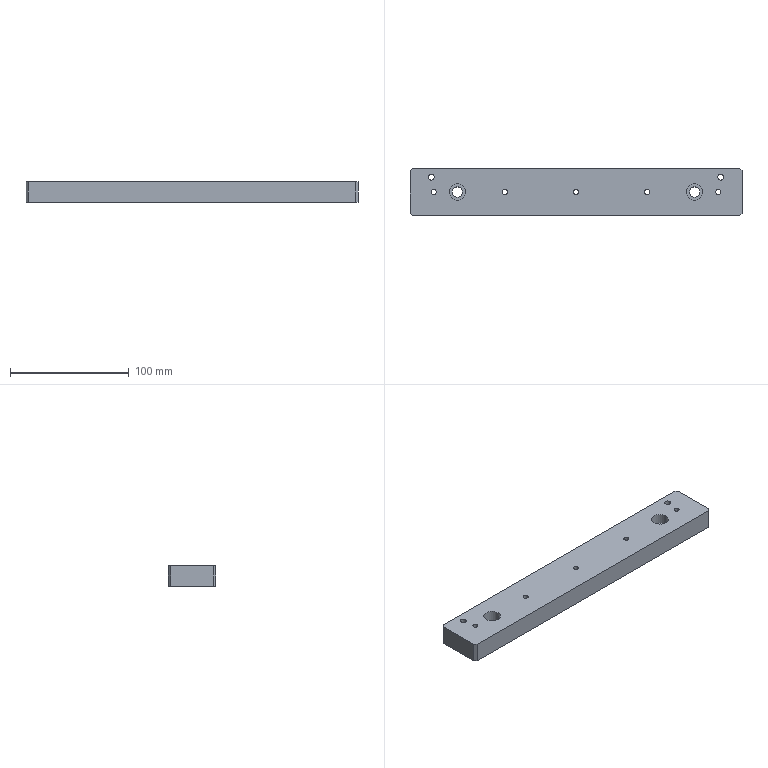Part | SolidWorks | features BaseBody 1 | 1 solid | 34 faces | box 280 x 40 x 17 mm | volume 184740 mm3 | cylinder 22 | plane 12 | commonest cylinder face diameters 4.2 x10 5 x4 8.5 x4 14 x4
STEP:
#1=CARTESIAN_POINT('',(-122.1,0.,0.));
#2=VERTEX_POINT('',#1);
#3=CARTESIAN_POINT('',(-117.9,0.,0.));
#4=VERTEX_POINT('',#3);
#5=CARTESIAN_POINT('',(-120.,0.,0.));
#6=DIRECTION('',(0.,0.,1.));
#7=DIRECTION('',(1.,0.,0.));
#8=AXIS2_PLACEMENT_3D('',#5,#6,#7);
#9=CIRCLE('',#8,2.1);
#10=EDGE_CURVE('',#2,#4,#9,.T.);
#11=ORIENTED_EDGE('',*,*,#10,.F.);
#12=CARTESIAN_POINT('',(-122.1,0.,17.));
#13=VERTEX_POINT('',#12);
#14=CARTESIAN_POINT('',(-122.1,0.,17.));
#15=DIRECTION('',(0.,0.,1.));
#16=VECTOR('',#15,1000.);
#17=LINE('',#14,#16);
#18=EDGE_CURVE('',#2,#13,#17,.T.);
#19=ORIENTED_EDGE('',*,*,#18,.T.);
#20=CARTESIAN_POINT('',(-117.9,0.,17.));
#21=VERTEX_POINT('',#20);
#22=CARTESIAN_POINT('',(-120.,0.,17.));
#23=DIRECTION('',(0.,0.,1.));
#24=DIRECTION('',(1.,0.,0.));
#25=AXIS2_PLACEMENT_3D('',#22,#23,#24);
#26=CIRCLE('',#25,2.1);
#27=EDGE_CURVE('',#13,#21,#26,.T.);
#28=ORIENTED_EDGE('',*,*,#27,.T.);
#29=CARTESIAN_POINT('',(-117.9,0.,17.));
#30=DIRECTION('',(0.,0.,1.));
#31=VECTOR('',#30,1000.);
#32=LINE('',#29,#31);
#33=EDGE_CURVE('',#4,#21,#32,.T.);
#34=ORIENTED_EDGE('',*,*,#33,.F.);
#35=EDGE_LOOP('',(#11,#19,#28,#34));
#36=FACE_OUTER_BOUND('',#35,.T.);
#37=CARTESIAN_POINT('',(-120.,0.,17.));
#38=DIRECTION('',(0.,0.,1.));
#39=DIRECTION('',(1.,0.,0.));
#40=AXIS2_PLACEMENT_3D('',#37,#38,#39);
#41=CYLINDRICAL_SURFACE('',#40,2.1);
#42=ADVANCED_FACE('',(#36),#41,.F.);
#43=CARTESIAN_POINT('',(-62.1,0.,0.));
#44=VERTEX_POINT('',#43);
#45=CARTESIAN_POINT('',(-57.9,0.,0.));
#46=VERTEX_POINT('',#45);
#47=CARTESIAN_POINT('',(-60.,0.,0.));
#48=DIRECTION('',(0.,0.,1.));
#49=DIRECTION('',(1.,0.,0.));
#50=AXIS2_PLACEMENT_3D('',#47,#48,#49);
#51=CIRCLE('',#50,2.1);
#52=EDGE_CURVE('',#44,#46,#51,.T.);
#53=ORIENTED_EDGE('',*,*,#52,.F.);
#54=CARTESIAN_POINT('',(-62.1,0.,17.));
#55=VERTEX_POINT('',#54);
#56=CARTESIAN_POINT('',(-62.1,0.,17.));
#57=DIRECTION('',(0.,0.,1.));
#58=VECTOR('',#57,1000.);
#59=LINE('',#56,#58);
#60=EDGE_CURVE('',#44,#55,#59,.T.);
#61=ORIENTED_EDGE('',*,*,#60,.T.);
#62=CARTESIAN_POINT('',(-57.9,0.,17.));
#63=VERTEX_POINT('',#62);
#64=CARTESIAN_POINT('',(-60.,0.,17.));
#65=DIRECTION('',(0.,0.,1.));
#66=DIRECTION('',(1.,0.,0.));
#67=AXIS2_PLACEMENT_3D('',#64,#65,#66);
#68=CIRCLE('',#67,2.1);
#69=EDGE_CURVE('',#55,#63,#68,.T.);
#70=ORIENTED_EDGE('',*,*,#69,.T.);
#71=CARTESIAN_POINT('',(-57.9,0.,17.));
#72=DIRECTION('',(0.,0.,1.));
#73=VECTOR('',#72,1000.);
#74=LINE('',#71,#73);
#75=EDGE_CURVE('',#46,#63,#74,.T.);
#76=ORIENTED_EDGE('',*,*,#75,.F.);
#77=EDGE_LOOP('',(#53,#61,#70,#76));
#78=FACE_OUTER_BOUND('',#77,.T.);
#79=CARTESIAN_POINT('',(-60.,0.,17.));
#80=DIRECTION('',(0.,0.,1.));
#81=DIRECTION('',(1.,0.,0.));
#82=AXIS2_PLACEMENT_3D('',#79,#80,#81);
#83=CYLINDRICAL_SURFACE('',#82,2.1);
#84=ADVANCED_FACE('',(#78),#83,.F.);
#85=CARTESIAN_POINT('',(-2.1,0.,0.));
#86=VERTEX_POINT('',#85);
#87=CARTESIAN_POINT('',(2.1,0.,0.));
#88=VERTEX_POINT('',#87);
#89=CARTESIAN_POINT('',(0.,0.,0.));
#90=DIRECTION('',(0.,0.,1.));
#91=DIRECTION('',(1.,0.,0.));
#92=AXIS2_PLACEMENT_3D('',#89,#90,#91);
#93=CIRCLE('',#92,2.1);
#94=EDGE_CURVE('',#86,#88,#93,.T.);
#95=ORIENTED_EDGE('',*,*,#94,.F.);
#96=CARTESIAN_POINT('',(-2.1,0.,17.));
#97=VERTEX_POINT('',#96);
#98=CARTESIAN_POINT('',(-2.1,0.,17.));
#99=DIRECTION('',(0.,0.,1.));
#100=VECTOR('',#99,1000.);
#101=LINE('',#98,#100);
#102=EDGE_CURVE('',#86,#97,#101,.T.);
#103=ORIENTED_EDGE('',*,*,#102,.T.);
#104=CARTESIAN_POINT('',(2.1,0.,17.));
#105=VERTEX_POINT('',#104);
#106=CARTESIAN_POINT('',(0.,0.,17.));
#107=DIRECTION('',(0.,0.,1.));
#108=DIRECTION('',(1.,0.,0.));
#109=AXIS2_PLACEMENT_3D('',#106,#107,#108);
#110=CIRCLE('',#109,2.1);
#111=EDGE_CURVE('',#97,#105,#110,.T.);
#112=ORIENTED_EDGE('',*,*,#111,.T.);
#113=CARTESIAN_POINT('',(2.1,0.,17.));
#114=DIRECTION('',(0.,0.,1.));
#115=VECTOR('',#114,1000.);
#116=LINE('',#113,#115);
#117=EDGE_CURVE('',#88,#105,#116,.T.);
#118=ORIENTED_EDGE('',*,*,#117,.F.);
#119=EDGE_LOOP('',(#95,#103,#112,#118));
#120=FACE_OUTER_BOUND('',#119,.T.);
#121=CARTESIAN_POINT('',(0.,0.,17.));
#122=DIRECTION('',(0.,0.,1.));
#123=DIRECTION('',(1.,0.,0.));
#124=AXIS2_PLACEMENT_3D('',#121,#122,#123);
#125=CYLINDRICAL_SURFACE('',#124,2.1);
#126=ADVANCED_FACE('',(#120),#125,.F.);
#127=CARTESIAN_POINT('',(57.9,0.,0.));
#128=VERTEX_POINT('',#127);
#129=CARTESIAN_POINT('',(62.1,0.,0.));
#130=VERTEX_POINT('',#129);
#131=CARTESIAN_POINT('',(60.,0.,0.));
#132=DIRECTION('',(0.,0.,1.));
#133=DIRECTION('',(1.,0.,0.));
#134=AXIS2_PLACEMENT_3D('',#131,#132,#133);
#135=CIRCLE('',#134,2.1);
#136=EDGE_CURVE('',#128,#130,#135,.T.);
#137=ORIENTED_EDGE('',*,*,#136,.F.);
#138=CARTESIAN_POINT('',(57.9,0.,17.));
#139=VERTEX_POINT('',#138);
#140=CARTESIAN_POINT('',(57.9,0.,17.));
#141=DIRECTION('',(0.,0.,1.));
#142=VECTOR('',#141,1000.);
#143=LINE('',#140,#142);
#144=EDGE_CURVE('',#128,#139,#143,.T.);
#145=ORIENTED_EDGE('',*,*,#144,.T.);
#146=CARTESIAN_POINT('',(62.1,0.,17.));
#147=VERTEX_POINT('',#146);
#148=CARTESIAN_POINT('',(60.,0.,17.));
#149=DIRECTION('',(0.,0.,1.));
#150=DIRECTION('',(1.,0.,0.));
#151=AXIS2_PLACEMENT_3D('',#148,#149,#150);
#152=CIRCLE('',#151,2.1);
#153=EDGE_CURVE('',#139,#147,#152,.T.);
#154=ORIENTED_EDGE('',*,*,#153,.T.);
#155=CARTESIAN_POINT('',(62.1,0.,17.));
#156=DIRECTION('',(0.,0.,1.));
#157=VECTOR('',#156,1000.);
#158=LINE('',#155,#157);
#159=EDGE_CURVE('',#130,#147,#158,.T.);
#160=ORIENTED_EDGE('',*,*,#159,.F.);
#161=EDGE_LOOP('',(#137,#145,#154,#160));
#162=FACE_OUTER_BOUND('',#161,.T.);
#163=CARTESIAN_POINT('',(60.,0.,17.));
#164=DIRECTION('',(0.,0.,1.));
#165=DIRECTION('',(1.,0.,0.));
#166=AXIS2_PLACEMENT_3D('',#163,#164,#165);
#167=CYLINDRICAL_SURFACE('',#166,2.1);
#168=ADVANCED_FACE('',(#162),#167,.F.);
#169=CARTESIAN_POINT('',(117.9,0.,0.));
#170=VERTEX_POINT('',#169);
#171=CARTESIAN_POINT('',(122.1,0.,0.));
#172=VERTEX_POINT('',#171);
#173=CARTESIAN_POINT('',(120.,0.,0.));
#174=DIRECTION('',(0.,0.,1.));
#175=DIRECTION('',(1.,0.,0.));
#176=AXIS2_PLACEMENT_3D('',#173,#174,#175);
#177=CIRCLE('',#176,2.1);
#178=EDGE_CURVE('',#170,#172,#177,.T.);
#179=ORIENTED_EDGE('',*,*,#178,.F.);
#180=CARTESIAN_POINT('',(117.9,0.,17.));
#181=VERTEX_POINT('',#180);
#182=CARTESIAN_POINT('',(117.9,0.,17.));
#183=DIRECTION('',(0.,0.,1.));
#184=VECTOR('',#183,1000.);
#185=LINE('',#182,#184);
#186=EDGE_CURVE('',#170,#181,#185,.T.);
#187=ORIENTED_EDGE('',*,*,#186,.T.);
#188=CARTESIAN_POINT('',(122.1,0.,17.));
#189=VERTEX_POINT('',#188);
#190=CARTESIAN_POINT('',(120.,0.,17.));
#191=DIRECTION('',(0.,0.,1.));
#192=DIRECTION('',(1.,0.,0.));
#193=AXIS2_PLACEMENT_3D('',#190,#191,#192);
#194=CIRCLE('',#193,2.1);
#195=EDGE_CURVE('',#181,#189,#194,.T.);
#196=ORIENTED_EDGE('',*,*,#195,.T.);
#197=CARTESIAN_POINT('',(122.1,0.,17.));
#198=DIRECTION('',(0.,0.,1.));
#199=VECTOR('',#198,1000.);
#200=LINE('',#197,#199);
#201=EDGE_CURVE('',#172,#189,#200,.T.);
#202=ORIENTED_EDGE('',*,*,#201,.F.);
#203=EDGE_LOOP('',(#179,#187,#196,#202));
#204=FACE_OUTER_BOUND('',#203,.T.);
#205=CARTESIAN_POINT('',(120.,0.,17.));
#206=DIRECTION('',(0.,0.,1.));
#207=DIRECTION('',(1.,0.,0.));
#208=AXIS2_PLACEMENT_3D('',#205,#206,#207);
#209=CYLINDRICAL_SURFACE('',#208,2.1);
#210=ADVANCED_FACE('',(#204),#209,.F.);
#211=CARTESIAN_POINT('',(-119.5,12.5,0.));
#212=VERTEX_POINT('',#211);
#213=CARTESIAN_POINT('',(-124.5,12.5,0.));
#214=VERTEX_POINT('',#213);
#215=CARTESIAN_POINT('',(-122.,12.5,0.));
#216=DIRECTION('',(0.,0.,-1.));
#217=DIRECTION('',(-1.,0.,0.));
#218=AXIS2_PLACEMENT_3D('',#215,#216,#217);
#219=CIRCLE('',#218,2.5);
#220=EDGE_CURVE('',#212,#214,#219,.T.);
#221=ORIENTED_EDGE('',*,*,#220,.T.);
#222=CARTESIAN_POINT('',(-124.5,12.5,17.));
#223=VERTEX_POINT('',#222);
#224=CARTESIAN_POINT('',(-124.5,12.5,17.));
#225=DIRECTION('',(0.,0.,1.));
#226=VECTOR('',#225,1000.);
#227=LINE('',#224,#226);
#228=EDGE_CURVE('',#214,#223,#227,.T.);
#229=ORIENTED_EDGE('',*,*,#228,.T.);
#230=CARTESIAN_POINT('',(-119.5,12.5,17.));
#231=VERTEX_POINT('',#230);
#232=CARTESIAN_POINT('',(-122.,12.5,17.));
#233=DIRECTION('',(0.,0.,1.));
#234=DIRECTION('',(1.,0.,0.));
#235=AXIS2_PLACEMENT_3D('',#232,#233,#234);
#236=CIRCLE('',#235,2.5);
#237=EDGE_CURVE('',#223,#231,#236,.T.);
#238=ORIENTED_EDGE('',*,*,#237,.T.);
#239=CARTESIAN_POINT('',(-119.5,12.5,17.));
#240=DIRECTION('',(0.,0.,1.));
#241=VECTOR('',#240,1000.);
#242=LINE('',#239,#241);
#243=EDGE_CURVE('',#212,#231,#242,.T.);
#244=ORIENTED_EDGE('',*,*,#243,.F.);
#245=EDGE_LOOP('',(#221,#229,#238,#244));
#246=FACE_OUTER_BOUND('',#245,.T.);
#247=CARTESIAN_POINT('',(-122.,12.5,17.));
#248=DIRECTION('',(0.,0.,1.));
#249=DIRECTION('',(1.,0.,0.));
#250=AXIS2_PLACEMENT_3D('',#247,#248,#249);
#251=CYLINDRICAL_SURFACE('',#250,2.5);
#252=ADVANCED_FACE('',(#246),#251,.F.);
#253=CARTESIAN_POINT('',(124.5,12.5,0.));
#254=VERTEX_POINT('',#253);
#255=CARTESIAN_POINT('',(119.5,12.5,0.));
#256=VERTEX_POINT('',#255);
#257=CARTESIAN_POINT('',(122.,12.5,0.));
#258=DIRECTION('',(0.,0.,-1.));
#259=DIRECTION('',(-1.,0.,0.));
#260=AXIS2_PLACEMENT_3D('',#257,#258,#259);
#261=CIRCLE('',#260,2.5);
#262=EDGE_CURVE('',#254,#256,#261,.T.);
#263=ORIENTED_EDGE('',*,*,#262,.T.);
#264=CARTESIAN_POINT('',(119.5,12.5,17.));
#265=VERTEX_POINT('',#264);
#266=CARTESIAN_POINT('',(119.5,12.5,17.));
#267=DIRECTION('',(0.,0.,1.));
#268=VECTOR('',#267,1000.);
#269=LINE('',#266,#268);
#270=EDGE_CURVE('',#256,#265,#269,.T.);
#271=ORIENTED_EDGE('',*,*,#270,.T.);
#272=CARTESIAN_POINT('',(124.5,12.5,17.));
#273=VERTEX_POINT('',#272);
#274=CARTESIAN_POINT('',(122.,12.5,17.));
#275=DIRECTION('',(0.,0.,1.));
#276=DIRECTION('',(1.,0.,0.));
#277=AXIS2_PLACEMENT_3D('',#274,#275,#276);
#278=CIRCLE('',#277,2.5);
#279=EDGE_CURVE('',#265,#273,#278,.T.);
#280=ORIENTED_EDGE('',*,*,#279,.T.);
#281=CARTESIAN_POINT('',(124.5,12.5,17.));
#282=DIRECTION('',(0.,0.,1.));
#283=VECTOR('',#282,1000.);
#284=LINE('',#281,#283);
#285=EDGE_CURVE('',#254,#273,#284,.T.);
#286=ORIENTED_EDGE('',*,*,#285,.F.);
#287=EDGE_LOOP('',(#263,#271,#280,#286));
#288=FACE_OUTER_BOUND('',#287,.T.);
#289=CARTESIAN_POINT('',(122.,12.5,17.));
#290=DIRECTION('',(0.,0.,1.));
#291=DIRECTION('',(1.,0.,0.));
#292=AXIS2_PLACEMENT_3D('',#289,#290,#291);
#293=CYLINDRICAL_SURFACE('',#292,2.5);
#294=ADVANCED_FACE('',(#288),#293,.F.);
#295=CARTESIAN_POINT('',(-107.,0.,8.));
#296=VERTEX_POINT('',#295);
#297=CARTESIAN_POINT('',(-93.,0.,8.));
#298=VERTEX_POINT('',#297);
#299=CARTESIAN_POINT('',(-100.,0.,8.));
#300=DIRECTION('',(0.,0.,1.));
#301=DIRECTION('',(1.,0.,0.));
#302=AXIS2_PLACEMENT_3D('',#299,#300,#301);
#303=CIRCLE('',#302,7.);
#304=EDGE_CURVE('',#296,#298,#303,.T.);
#305=ORIENTED_EDGE('',*,*,#304,.F.);
#306=CARTESIAN_POINT('',(-107.,0.,17.));
#307=VERTEX_POINT('',#306);
#308=CARTESIAN_POINT('',(-107.,0.,17.));
#309=DIRECTION('',(0.,0.,1.));
#310=VECTOR('',#309,1000.);
#311=LINE('',#308,#310);
#312=EDGE_CURVE('',#296,#307,#311,.T.);
#313=ORIENTED_EDGE('',*,*,#312,.T.);
#314=CARTESIAN_POINT('',(-93.,0.,17.));
#315=VERTEX_POINT('',#314);
#316=CARTESIAN_POINT('',(-100.,0.,17.));
#317=DIRECTION('',(0.,0.,1.));
#318=DIRECTION('',(1.,0.,0.));
#319=AXIS2_PLACEMENT_3D('',#316,#317,#318);
#320=CIRCLE('',#319,7.);
#321=EDGE_CURVE('',#307,#315,#320,.T.);
#322=ORIENTED_EDGE('',*,*,#321,.T.);
#323=CARTESIAN_POINT('',(-93.,0.,17.));
#324=DIRECTION('',(0.,0.,1.));
#325=VECTOR('',#324,1000.);
#326=LINE('',#323,#325);
#327=EDGE_CURVE('',#298,#315,#326,.T.);
#328=ORIENTED_EDGE('',*,*,#327,.F.);
#329=EDGE_LOOP('',(#305,#313,#322,#328));
#330=FACE_OUTER_BOUND('',#329,.T.);
#331=CARTESIAN_POINT('',(-100.,0.,17.));
#332=DIRECTION('',(0.,0.,1.));
#333=DIRECTION('',(1.,0.,0.));
#334=AXIS2_PLACEMENT_3D('',#331,#332,#333);
#335=CYLINDRICAL_SURFACE('',#334,7.);
#336=ADVANCED_FACE('',(#330),#335,.F.);
#337=CARTESIAN_POINT('',(-104.25,0.,0.));
#338=VERTEX_POINT('',#337);
#339=CARTESIAN_POINT('',(-95.75,0.,0.));
#340=VERTEX_POINT('',#339);
#341=CARTESIAN_POINT('',(-100.,0.,0.));
#342=DIRECTION('',(0.,0.,1.));
#343=DIRECTION('',(1.,0.,0.));
#344=AXIS2_PLACEMENT_3D('',#341,#342,#343);
#345=CIRCLE('',#344,4.25);
#346=EDGE_CURVE('',#338,#340,#345,.T.);
#347=ORIENTED_EDGE('',*,*,#346,.F.);
#348=CARTESIAN_POINT('',(-104.25,0.,8.));
#349=VERTEX_POINT('',#348);
#350=CARTESIAN_POINT('',(-104.25,0.,17.));
#351=DIRECTION('',(0.,0.,1.));
#352=VECTOR('',#351,1000.);
#353=LINE('',#350,#352);
#354=EDGE_CURVE('',#338,#349,#353,.T.);
#355=ORIENTED_EDGE('',*,*,#354,.T.);
#356=CARTESIAN_POINT('',(-95.75,0.,8.));
#357=VERTEX_POINT('',#356);
#358=CARTESIAN_POINT('',(-100.,0.,8.));
#359=DIRECTION('',(0.,0.,1.));
#360=DIRECTION('',(1.,0.,0.));
#361=AXIS2_PLACEMENT_3D('',#358,#359,#360);
#362=CIRCLE('',#361,4.25);
#363=EDGE_CURVE('',#349,#357,#362,.T.);
#364=ORIENTED_EDGE('',*,*,#363,.T.);
#365=CARTESIAN_POINT('',(-95.75,0.,17.));
#366=DIRECTION('',(0.,0.,1.));
#367=VECTOR('',#366,1000.);
#368=LINE('',#365,#367);
#369=EDGE_CURVE('',#340,#357,#368,.T.);
#370=ORIENTED_EDGE('',*,*,#369,.F.);
#371=EDGE_LOOP('',(#347,#355,#364,#370));
#372=FACE_OUTER_BOUND('',#371,.T.);
#373=CARTESIAN_POINT('',(-100.,0.,17.));
#374=DIRECTION('',(0.,0.,1.));
#375=DIRECTION('',(1.,0.,0.));
#376=AXIS2_PLACEMENT_3D('',#373,#374,#375);
#377=CYLINDRICAL_SURFACE('',#376,4.25);
#378=ADVANCED_FACE('',(#372),#377,.F.);
#379=CARTESIAN_POINT('',(93.,0.,8.));
#380=VERTEX_POINT('',#379);
#381=CARTESIAN_POINT('',(107.,0.,8.));
#382=VERTEX_POINT('',#381);
#383=CARTESIAN_POINT('',(100.,0.,8.));
#384=DIRECTION('',(0.,0.,1.));
#385=DIRECTION('',(1.,0.,0.));
#386=AXIS2_PLACEMENT_3D('',#383,#384,#385);
#387=CIRCLE('',#386,7.);
#388=EDGE_CURVE('',#380,#382,#387,.T.);
#389=ORIENTED_EDGE('',*,*,#388,.F.);
#390=CARTESIAN_POINT('',(93.,0.,17.));
#391=VERTEX_POINT('',#390);
#392=CARTESIAN_POINT('',(93.,0.,17.));
#393=DIRECTION('',(0.,0.,1.));
#394=VECTOR('',#393,1000.);
#395=LINE('',#392,#394);
#396=EDGE_CURVE('',#380,#391,#395,.T.);
#397=ORIENTED_EDGE('',*,*,#396,.T.);
#398=CARTESIAN_POINT('',(107.,0.,17.));
#399=VERTEX_POINT('',#398);
#400=CARTESIAN_POINT('',(100.,0.,17.));
#401=DIRECTION('',(0.,0.,1.));
#402=DIRECTION('',(1.,0.,0.));
#403=AXIS2_PLACEMENT_3D('',#400,#401,#402);
#404=CIRCLE('',#403,7.);
#405=EDGE_CURVE('',#391,#399,#404,.T.);
#406=ORIENTED_EDGE('',*,*,#405,.T.);
#407=CARTESIAN_POINT('',(107.,0.,17.));
#408=DIRECTION('',(0.,0.,1.));
#409=VECTOR('',#408,1000.);
#410=LINE('',#407,#409);
#411=EDGE_CURVE('',#382,#399,#410,.T.);
#412=ORIENTED_EDGE('',*,*,#411,.F.);
#413=EDGE_LOOP('',(#389,#397,#406,#412));
#414=FACE_OUTER_BOUND('',#413,.T.);
#415=CARTESIAN_POINT('',(100.,0.,17.));
#416=DIRECTION('',(0.,0.,1.));
#417=DIRECTION('',(1.,0.,0.));
#418=AXIS2_PLACEMENT_3D('',#415,#416,#417);
#419=CYLINDRICAL_SURFACE('',#418,7.);
#420=ADVANCED_FACE('',(#414),#419,.F.);
#421=CARTESIAN_POINT('',(95.75,0.,0.));
#422=VERTEX_POINT('',#421);
#423=CARTESIAN_POINT('',(104.25,0.,0.));
#424=VERTEX_POINT('',#423);
#425=CARTESIAN_POINT('',(100.,0.,0.));
#426=DIRECTION('',(0.,0.,1.));
#427=DIRECTION('',(1.,0.,0.));
#428=AXIS2_PLACEMENT_3D('',#425,#426,#427);
#429=CIRCLE('',#428,4.25);
#430=EDGE_CURVE('',#422,#424,#429,.T.);
#431=ORIENTED_EDGE('',*,*,#430,.F.);
#432=CARTESIAN_POINT('',(95.75,0.,8.));
#433=VERTEX_POINT('',#432);
#434=CARTESIAN_POINT('',(95.75,0.,17.));
#435=DIRECTION('',(0.,0.,1.));
#436=VECTOR('',#435,1000.);
#437=LINE('',#434,#436);
#438=EDGE_CURVE('',#422,#433,#437,.T.);
#439=ORIENTED_EDGE('',*,*,#438,.T.);
#440=CARTESIAN_POINT('',(104.25,0.,8.));
#441=VERTEX_POINT('',#440);
#442=CARTESIAN_POINT('',(100.,0.,8.));
#443=DIRECTION('',(0.,0.,1.));
#444=DIRECTION('',(1.,0.,0.));
#445=AXIS2_PLACEMENT_3D('',#442,#443,#444);
#446=CIRCLE('',#445,4.25);
#447=EDGE_CURVE('',#433,#441,#446,.T.);
#448=ORIENTED_EDGE('',*,*,#447,.T.);
#449=CARTESIAN_POINT('',(104.25,0.,17.));
#450=DIRECTION('',(0.,0.,1.));
#451=VECTOR('',#450,1000.);
#452=LINE('',#449,#451);
#453=EDGE_CURVE('',#424,#441,#452,.T.);
#454=ORIENTED_EDGE('',*,*,#453,.F.);
#455=EDGE_LOOP('',(#431,#439,#448,#454));
#456=FACE_OUTER_BOUND('',#455,.T.);
#457=CARTESIAN_POINT('',(100.,0.,17.));
#458=DIRECTION('',(0.,0.,1.));
#459=DIRECTION('',(1.,0.,0.));
#460=AXIS2_PLACEMENT_3D('',#457,#458,#459);
#461=CYLINDRICAL_SURFACE('',#460,4.25);
#462=ADVANCED_FACE('',(#456),#461,.F.);
#463=CARTESIAN_POINT('',(-140.,18.,17.));
#464=VERTEX_POINT('',#463);
#465=CARTESIAN_POINT('',(-140.,-18.,17.));
#466=VERTEX_POINT('',#465);
#467=CARTESIAN_POINT('',(-140.,20.,17.));
#468=DIRECTION('',(0.,-1.,0.));
#469=VECTOR('',#468,1000.);
#470=LINE('',#467,#469);
#471=EDGE_CURVE('',#464,#466,#470,.T.);
#472=ORIENTED_EDGE('',*,*,#471,.F.);
#473=CARTESIAN_POINT('',(-140.,18.,0.));
#474=VERTEX_POINT('',#473);
#475=CARTESIAN_POINT('',(-140.,18.,17.));
#476=DIRECTION('',(0.,0.,-1.));
#477=VECTOR('',#476,1000.);
#478=LINE('',#475,#477);
#479=EDGE_CURVE('',#464,#474,#478,.T.);
#480=ORIENTED_EDGE('',*,*,#479,.T.);
#481=CARTESIAN_POINT('',(-140.,-18.,0.));
#482=VERTEX_POINT('',#481);
#483=CARTESIAN_POINT('',(-140.,20.,0.));
#484=DIRECTION('',(0.,-1.,0.));
#485=VECTOR('',#484,1000.);
#486=LINE('',#483,#485);
#487=EDGE_CURVE('',#474,#482,#486,.T.);
#488=ORIENTED_EDGE('',*,*,#487,.T.);
#489=CARTESIAN_POINT('',(-140.,-18.,17.));
#490=DIRECTION('',(0.,0.,1.));
#491=VECTOR('',#490,1000.);
#492=LINE('',#489,#491);
#493=EDGE_CURVE('',#482,#466,#492,.T.);
#494=ORIENTED_EDGE('',*,*,#493,.T.);
#495=EDGE_LOOP('',(#472,#480,#488,#494));
#496=FACE_OUTER_BOUND('',#495,.T.);
#497=CARTESIAN_POINT('',(-140.,20.,17.));
#498=DIRECTION('',(1.,0.,0.));
#499=DIRECTION('',(0.,0.,-1.));
#500=AXIS2_PLACEMENT_3D('',#497,#498,#499);
#501=PLANE('',#500);
#502=ADVANCED_FACE('',(#496),#501,.F.);
#503=CARTESIAN_POINT('',(-138.,-20.,0.));
#504=VERTEX_POINT('',#503);
#505=CARTESIAN_POINT('',(138.,-20.,0.));
#506=VERTEX_POINT('',#505);
#507=CARTESIAN_POINT('',(140.,-20.,0.));
#508=DIRECTION('',(1.,0.,0.));
#509=VECTOR('',#508,1000.);
#510=LINE('',#507,#509);
#511=EDGE_CURVE('',#504,#506,#510,.T.);
#512=ORIENTED_EDGE('',*,*,#511,.T.);
#513=CARTESIAN_POINT('',(138.,-20.,17.));
#514=VERTEX_POINT('',#513);
#515=CARTESIAN_POINT('',(138.,-20.,17.));
#516=DIRECTION('',(0.,0.,1.));
#517=VECTOR('',#516,1000.);
#518=LINE('',#515,#517);
#519=EDGE_CURVE('',#506,#514,#518,.T.);
#520=ORIENTED_EDGE('',*,*,#519,.T.);
#521=CARTESIAN_POINT('',(-138.,-20.,17.));
#522=VERTEX_POINT('',#521);
#523=CARTESIAN_POINT('',(140.,-20.,17.));
#524=DIRECTION('',(1.,0.,0.));
#525=VECTOR('',#524,1000.);
#526=LINE('',#523,#525);
#527=EDGE_CURVE('',#522,#514,#526,.T.);
#528=ORIENTED_EDGE('',*,*,#527,.F.);
#529=CARTESIAN_POINT('',(-138.,-20.,17.));
#530=DIRECTION('',(0.,0.,-1.));
#531=VECTOR('',#530,1000.);
#532=LINE('',#529,#531);
#533=EDGE_CURVE('',#522,#504,#532,.T.);
#534=ORIENTED_EDGE('',*,*,#533,.T.);
#535=EDGE_LOOP('',(#512,#520,#528,#534));
#536=FACE_OUTER_BOUND('',#535,.T.);
#537=CARTESIAN_POINT('',(140.,-20.,17.));
#538=DIRECTION('',(0.,1.,0.));
#539=DIRECTION('',(-1.,0.,0.));
#540=AXIS2_PLACEMENT_3D('',#537,#538,#539);
#541=PLANE('',#540);
#542=ADVANCED_FACE('',(#536),#541,.F.);
#543=CARTESIAN_POINT('',(140.,-18.,17.));
#544=VERTEX_POINT('',#543);
#545=CARTESIAN_POINT('',(140.,18.,17.));
#546=VERTEX_POINT('',#545);
#547=CARTESIAN_POINT('',(140.,20.,17.));
#548=DIRECTION('',(0.,1.,0.));
#549=VECTOR('',#548,1000.);
#550=LINE('',#547,#549);
#551=EDGE_CURVE('',#544,#546,#550,.T.);
#552=ORIENTED_EDGE('',*,*,#551,.F.);
#553=CARTESIAN_POINT('',(140.,-18.,0.));
#554=VERTEX_POINT('',#553);
#555=CARTESIAN_POINT('',(140.,-18.,17.));
#556=DIRECTION('',(0.,0.,-1.));
#557=VECTOR('',#556,1000.);
#558=LINE('',#555,#557);
#559=EDGE_CURVE('',#544,#554,#558,.T.);
#560=ORIENTED_EDGE('',*,*,#559,.T.);
#561=CARTESIAN_POINT('',(140.,18.,0.));
#562=VERTEX_POINT('',#561);
#563=CARTESIAN_POINT('',(140.,20.,0.));
#564=DIRECTION('',(0.,1.,0.));
#565=VECTOR('',#564,1000.);
#566=LINE('',#563,#565);
#567=EDGE_CURVE('',#554,#562,#566,.T.);
#568=ORIENTED_EDGE('',*,*,#567,.T.);
#569=CARTESIAN_POINT('',(140.,18.,17.));
#570=DIRECTION('',(0.,0.,1.));
#571=VECTOR('',#570,1000.);
#572=LINE('',#569,#571);
#573=EDGE_CURVE('',#562,#546,#572,.T.);
#574=ORIENTED_EDGE('',*,*,#573,.T.);
#575=EDGE_LOOP('',(#552,#560,#568,#574));
#576=FACE_OUTER_BOUND('',#575,.T.);
#577=CARTESIAN_POINT('',(140.,20.,17.));
#578=DIRECTION('',(-1.,0.,0.));
#579=DIRECTION('',(0.,0.,1.));
#580=AXIS2_PLACEMENT_3D('',#577,#578,#579);
#581=PLANE('',#580);
#582=ADVANCED_FACE('',(#576),#581,.F.);
#583=CARTESIAN_POINT('',(138.,20.,17.));
#584=VERTEX_POINT('',#583);
#585=CARTESIAN_POINT('',(-138.,20.,17.));
#586=VERTEX_POINT('',#585);
#587=CARTESIAN_POINT('',(140.,20.,17.));
#588=DIRECTION('',(-1.,0.,0.));
#589=VECTOR('',#588,1000.);
#590=LINE('',#587,#589);
#591=EDGE_CURVE('',#584,#586,#590,.T.);
#592=ORIENTED_EDGE('',*,*,#591,.F.);
#593=CARTESIAN_POINT('',(138.,20.,0.));
#594=VERTEX_POINT('',#593);
#595=CARTESIAN_POINT('',(138.,20.,17.));
#596=DIRECTION('',(0.,0.,-1.));
#597=VECTOR('',#596,1000.);
#598=LINE('',#595,#597);
#599=EDGE_CURVE('',#584,#594,#598,.T.);
#600=ORIENTED_EDGE('',*,*,#599,.T.);
#601=CARTESIAN_POINT('',(-138.,20.,0.));
#602=VERTEX_POINT('',#601);
#603=CARTESIAN_POINT('',(140.,20.,0.));
#604=DIRECTION('',(-1.,0.,0.));
#605=VECTOR('',#604,1000.);
#606=LINE('',#603,#605);
#607=EDGE_CURVE('',#594,#602,#606,.T.);
#608=ORIENTED_EDGE('',*,*,#607,.T.);
#609=CARTESIAN_POINT('',(-138.,20.,17.));
#610=DIRECTION('',(0.,0.,1.));
#611=VECTOR('',#610,1000.);
#612=LINE('',#609,#611);
#613=EDGE_CURVE('',#602,#586,#612,.T.);
#614=ORIENTED_EDGE('',*,*,#613,.T.);
#615=EDGE_LOOP('',(#592,#600,#608,#614));
#616=FACE_OUTER_BOUND('',#615,.T.);
#617=CARTESIAN_POINT('',(140.,20.,17.));
#618=DIRECTION('',(0.,-1.,0.));
#619=DIRECTION('',(1.,0.,0.));
#620=AXIS2_PLACEMENT_3D('',#617,#618,#619);
#621=PLANE('',#620);
#622=ADVANCED_FACE('',(#616),#621,.F.);
#623=CARTESIAN_POINT('',(-120.,0.,17.));
#624=DIRECTION('',(0.,0.,1.));
#625=DIRECTION('',(1.,0.,0.));
#626=AXIS2_PLACEMENT_3D('',#623,#624,#625);
#627=CIRCLE('',#626,2.1);
#628=EDGE_CURVE('',#21,#13,#627,.T.);
#629=ORIENTED_EDGE('',*,*,#628,.F.);
#630=ORIENTED_EDGE('',*,*,#27,.F.);
#631=EDGE_LOOP('',(#629,#630));
#632=FACE_BOUND('',#631,.T.);
#633=CARTESIAN_POINT('',(-60.,0.,17.));
#634=DIRECTION('',(0.,0.,1.));
#635=DIRECTION('',(1.,0.,0.));
#636=AXIS2_PLACEMENT_3D('',#633,#634,#635);
#637=CIRCLE('',#636,2.1);
#638=EDGE_CURVE('',#63,#55,#637,.T.);
#639=ORIENTED_EDGE('',*,*,#638,.F.);
#640=ORIENTED_EDGE('',*,*,#69,.F.);
#641=EDGE_LOOP('',(#639,#640));
#642=FACE_BOUND('',#641,.T.);
#643=CARTESIAN_POINT('',(0.,0.,17.));
#644=DIRECTION('',(0.,0.,1.));
#645=DIRECTION('',(1.,0.,0.));
#646=AXIS2_PLACEMENT_3D('',#643,#644,#645);
#647=CIRCLE('',#646,2.1);
#648=EDGE_CURVE('',#105,#97,#647,.T.);
#649=ORIENTED_EDGE('',*,*,#648,.F.);
#650=ORIENTED_EDGE('',*,*,#111,.F.);
#651=EDGE_LOOP('',(#649,#650));
#652=FACE_BOUND('',#651,.T.);
#653=CARTESIAN_POINT('',(60.,0.,17.));
#654=DIRECTION('',(0.,0.,1.));
#655=DIRECTION('',(1.,0.,0.));
#656=AXIS2_PLACEMENT_3D('',#653,#654,#655);
#657=CIRCLE('',#656,2.1);
#658=EDGE_CURVE('',#147,#139,#657,.T.);
#659=ORIENTED_EDGE('',*,*,#658,.F.);
#660=ORIENTED_EDGE('',*,*,#153,.F.);
#661=EDGE_LOOP('',(#659,#660));
#662=FACE_BOUND('',#661,.T.);
#663=CARTESIAN_POINT('',(120.,0.,17.));
#664=DIRECTION('',(0.,0.,1.));
#665=DIRECTION('',(1.,0.,0.));
#666=AXIS2_PLACEMENT_3D('',#663,#664,#665);
#667=CIRCLE('',#666,2.1);
#668=EDGE_CURVE('',#189,#181,#667,.T.);
#669=ORIENTED_EDGE('',*,*,#668,.F.);
#670=ORIENTED_EDGE('',*,*,#195,.F.);
#671=EDGE_LOOP('',(#669,#670));
#672=FACE_BOUND('',#671,.T.);
#673=CARTESIAN_POINT('',(-122.,12.5,17.));
#674=DIRECTION('',(0.,0.,1.));
#675=DIRECTION('',(1.,0.,0.));
#676=AXIS2_PLACEMENT_3D('',#673,#674,#675);
#677=CIRCLE('',#676,2.5);
#678=EDGE_CURVE('',#231,#223,#677,.T.);
#679=ORIENTED_EDGE('',*,*,#678,.F.);
#680=ORIENTED_EDGE('',*,*,#237,.F.);
#681=EDGE_LOOP('',(#679,#680));
#682=FACE_BOUND('',#681,.T.);
#683=CARTESIAN_POINT('',(122.,12.5,17.));
#684=DIRECTION('',(0.,0.,1.));
#685=DIRECTION('',(1.,0.,0.));
#686=AXIS2_PLACEMENT_3D('',#683,#684,#685);
#687=CIRCLE('',#686,2.5);
#688=EDGE_CURVE('',#273,#265,#687,.T.);
#689=ORIENTED_EDGE('',*,*,#688,.F.);
#690=ORIENTED_EDGE('',*,*,#279,.F.);
#691=EDGE_LOOP('',(#689,#690));
#692=FACE_BOUND('',#691,.T.);
#693=CARTESIAN_POINT('',(-100.,0.,17.));
#694=DIRECTION('',(0.,0.,1.));
#695=DIRECTION('',(1.,0.,0.));
#696=AXIS2_PLACEMENT_3D('',#693,#694,#695);
#697=CIRCLE('',#696,7.);
#698=EDGE_CURVE('',#315,#307,#697,.T.);
#699=ORIENTED_EDGE('',*,*,#698,.F.);
#700=ORIENTED_EDGE('',*,*,#321,.F.);
#701=EDGE_LOOP('',(#699,#700));
#702=FACE_BOUND('',#701,.T.);
#703=CARTESIAN_POINT('',(100.,0.,17.));
#704=DIRECTION('',(0.,0.,1.));
#705=DIRECTION('',(1.,0.,0.));
#706=AXIS2_PLACEMENT_3D('',#703,#704,#705);
#707=CIRCLE('',#706,7.);
#708=EDGE_CURVE('',#399,#391,#707,.T.);
#709=ORIENTED_EDGE('',*,*,#708,.F.);
#710=ORIENTED_EDGE('',*,*,#405,.F.);
#711=EDGE_LOOP('',(#709,#710));
#712=FACE_BOUND('',#711,.T.);
#713=ORIENTED_EDGE('',*,*,#527,.T.);
#714=CARTESIAN_POINT('',(140.,-18.,17.));
#715=DIRECTION('',(0.7071,0.7071,0.));
#716=VECTOR('',#715,1000.);
#717=LINE('',#714,#716);
#718=EDGE_CURVE('',#514,#544,#717,.T.);
#719=ORIENTED_EDGE('',*,*,#718,.T.);
#720=ORIENTED_EDGE('',*,*,#551,.T.);
#721=CARTESIAN_POINT('',(138.,20.,17.));
#722=DIRECTION('',(-0.7071,0.7071,0.));
#723=VECTOR('',#722,1000.);
#724=LINE('',#721,#723);
#725=EDGE_CURVE('',#546,#584,#724,.T.);
#726=ORIENTED_EDGE('',*,*,#725,.T.);
#727=ORIENTED_EDGE('',*,*,#591,.T.);
#728=CARTESIAN_POINT('',(-140.,18.,17.));
#729=DIRECTION('',(-0.7071,-0.7071,0.));
#730=VECTOR('',#729,1000.);
#731=LINE('',#728,#730);
#732=EDGE_CURVE('',#586,#464,#731,.T.);
#733=ORIENTED_EDGE('',*,*,#732,.T.);
#734=ORIENTED_EDGE('',*,*,#471,.T.);
#735=CARTESIAN_POINT('',(-138.,-20.,17.));
#736=DIRECTION('',(0.7071,-0.7071,0.));
#737=VECTOR('',#736,1000.);
#738=LINE('',#735,#737);
#739=EDGE_CURVE('',#466,#522,#738,.T.);
#740=ORIENTED_EDGE('',*,*,#739,.T.);
#741=EDGE_LOOP('',(#713,#719,#720,#726,#727,#733,#734,#740));
#742=FACE_OUTER_BOUND('',#741,.T.);
#743=CARTESIAN_POINT('',(-140.,-20.,17.));
#744=DIRECTION('',(0.,0.,-1.));
#745=DIRECTION('',(-1.,0.,0.));
#746=AXIS2_PLACEMENT_3D('',#743,#744,#745);
#747=PLANE('',#746);
#748=ADVANCED_FACE('',(#632,#642,#652,#662,#672,#682,#692,#702,#712,#742),#747,.F.);
#749=CARTESIAN_POINT('',(-120.,0.,0.));
#750=DIRECTION('',(0.,0.,1.));
#751=DIRECTION('',(1.,0.,0.));
#752=AXIS2_PLACEMENT_3D('',#749,#750,#751);
#753=CIRCLE('',#752,2.1);
#754=EDGE_CURVE('',#4,#2,#753,.T.);
#755=ORIENTED_EDGE('',*,*,#754,.T.);
#756=ORIENTED_EDGE('',*,*,#10,.T.);
#757=EDGE_LOOP('',(#755,#756));
#758=FACE_BOUND('',#757,.T.);
#759=CARTESIAN_POINT('',(-60.,0.,0.));
#760=DIRECTION('',(0.,0.,1.));
#761=DIRECTION('',(1.,0.,0.));
#762=AXIS2_PLACEMENT_3D('',#759,#760,#761);
#763=CIRCLE('',#762,2.1);
#764=EDGE_CURVE('',#46,#44,#763,.T.);
#765=ORIENTED_EDGE('',*,*,#764,.T.);
#766=ORIENTED_EDGE('',*,*,#52,.T.);
#767=EDGE_LOOP('',(#765,#766));
#768=FACE_BOUND('',#767,.T.);
#769=CARTESIAN_POINT('',(0.,0.,0.));
#770=DIRECTION('',(0.,0.,1.));
#771=DIRECTION('',(1.,0.,0.));
#772=AXIS2_PLACEMENT_3D('',#769,#770,#771);
#773=CIRCLE('',#772,2.1);
#774=EDGE_CURVE('',#88,#86,#773,.T.);
#775=ORIENTED_EDGE('',*,*,#774,.T.);
#776=ORIENTED_EDGE('',*,*,#94,.T.);
#777=EDGE_LOOP('',(#775,#776));
#778=FACE_BOUND('',#777,.T.);
#779=CARTESIAN_POINT('',(60.,0.,0.));
#780=DIRECTION('',(0.,0.,1.));
#781=DIRECTION('',(1.,0.,0.));
#782=AXIS2_PLACEMENT_3D('',#779,#780,#781);
#783=CIRCLE('',#782,2.1);
#784=EDGE_CURVE('',#130,#128,#783,.T.);
#785=ORIENTED_EDGE('',*,*,#784,.T.);
#786=ORIENTED_EDGE('',*,*,#136,.T.);
#787=EDGE_LOOP('',(#785,#786));
#788=FACE_BOUND('',#787,.T.);
#789=CARTESIAN_POINT('',(120.,0.,0.));
#790=DIRECTION('',(0.,0.,1.));
#791=DIRECTION('',(1.,0.,0.));
#792=AXIS2_PLACEMENT_3D('',#789,#790,#791);
#793=CIRCLE('',#792,2.1);
#794=EDGE_CURVE('',#172,#170,#793,.T.);
#795=ORIENTED_EDGE('',*,*,#794,.T.);
#796=ORIENTED_EDGE('',*,*,#178,.T.);
#797=EDGE_LOOP('',(#795,#796));
#798=FACE_BOUND('',#797,.T.);
#799=ORIENTED_EDGE('',*,*,#220,.F.);
#800=CARTESIAN_POINT('',(-122.,12.5,0.));
#801=DIRECTION('',(0.,0.,-1.));
#802=DIRECTION('',(-1.,0.,0.));
#803=AXIS2_PLACEMENT_3D('',#800,#801,#802);
#804=CIRCLE('',#803,2.5);
#805=EDGE_CURVE('',#214,#212,#804,.T.);
#806=ORIENTED_EDGE('',*,*,#805,.F.);
#807=EDGE_LOOP('',(#799,#806));
#808=FACE_BOUND('',#807,.T.);
#809=ORIENTED_EDGE('',*,*,#262,.F.);
#810=CARTESIAN_POINT('',(122.,12.5,0.));
#811=DIRECTION('',(0.,0.,-1.));
#812=DIRECTION('',(-1.,0.,0.));
#813=AXIS2_PLACEMENT_3D('',#810,#811,#812);
#814=CIRCLE('',#813,2.5);
#815=EDGE_CURVE('',#256,#254,#814,.T.);
#816=ORIENTED_EDGE('',*,*,#815,.F.);
#817=EDGE_LOOP('',(#809,#816));
#818=FACE_BOUND('',#817,.T.);
#819=CARTESIAN_POINT('',(-100.,0.,0.));
#820=DIRECTION('',(0.,0.,1.));
#821=DIRECTION('',(1.,0.,0.));
#822=AXIS2_PLACEMENT_3D('',#819,#820,#821);
#823=CIRCLE('',#822,4.25);
#824=EDGE_CURVE('',#340,#338,#823,.T.);
#825=ORIENTED_EDGE('',*,*,#824,.T.);
#826=ORIENTED_EDGE('',*,*,#346,.T.);
#827=EDGE_LOOP('',(#825,#826));
#828=FACE_BOUND('',#827,.T.);
#829=CARTESIAN_POINT('',(100.,0.,0.));
#830=DIRECTION('',(0.,0.,1.));
#831=DIRECTION('',(1.,0.,0.));
#832=AXIS2_PLACEMENT_3D('',#829,#830,#831);
#833=CIRCLE('',#832,4.25);
#834=EDGE_CURVE('',#424,#422,#833,.T.);
#835=ORIENTED_EDGE('',*,*,#834,.T.);
#836=ORIENTED_EDGE('',*,*,#430,.T.);
#837=EDGE_LOOP('',(#835,#836));
#838=FACE_BOUND('',#837,.T.);
#839=ORIENTED_EDGE('',*,*,#567,.F.);
#840=CARTESIAN_POINT('',(-1.,-159.,0.));
#841=DIRECTION('',(-0.7071,-0.7071,0.));
#842=VECTOR('',#841,1000.);
#843=LINE('',#840,#842);
#844=EDGE_CURVE('',#554,#506,#843,.T.);
#845=ORIENTED_EDGE('',*,*,#844,.T.);
#846=ORIENTED_EDGE('',*,*,#511,.F.);
#847=CARTESIAN_POINT('',(-139.,-19.,0.));
#848=DIRECTION('',(-0.7071,0.7071,0.));
#849=VECTOR('',#848,1000.);
#850=LINE('',#847,#849);
#851=EDGE_CURVE('',#504,#482,#850,.T.);
#852=ORIENTED_EDGE('',*,*,#851,.T.);
#853=ORIENTED_EDGE('',*,*,#487,.F.);
#854=CARTESIAN_POINT('',(-159.,-1.,0.));
#855=DIRECTION('',(0.7071,0.7071,0.));
#856=VECTOR('',#855,1000.);
#857=LINE('',#854,#856);
#858=EDGE_CURVE('',#474,#602,#857,.T.);
#859=ORIENTED_EDGE('',*,*,#858,.T.);
#860=ORIENTED_EDGE('',*,*,#607,.F.);
#861=CARTESIAN_POINT('',(19.,139.,0.));
#862=DIRECTION('',(0.7071,-0.7071,0.));
#863=VECTOR('',#862,1000.);
#864=LINE('',#861,#863);
#865=EDGE_CURVE('',#594,#562,#864,.T.);
#866=ORIENTED_EDGE('',*,*,#865,.T.);
#867=EDGE_LOOP('',(#839,#845,#846,#852,#853,#859,#860,#866));
#868=FACE_OUTER_BOUND('',#867,.T.);
#869=CARTESIAN_POINT('',(-140.,-20.,0.));
#870=DIRECTION('',(0.,0.,-1.));
#871=DIRECTION('',(-1.,0.,0.));
#872=AXIS2_PLACEMENT_3D('',#869,#870,#871);
#873=PLANE('',#872);
#874=ADVANCED_FACE('',(#758,#768,#778,#788,#798,#808,#818,#828,#838,#868),#873,.T.);
#875=ORIENTED_EDGE('',*,*,#438,.F.);
#876=ORIENTED_EDGE('',*,*,#834,.F.);
#877=ORIENTED_EDGE('',*,*,#453,.T.);
#878=CARTESIAN_POINT('',(100.,0.,8.));
#879=DIRECTION('',(0.,0.,1.));
#880=DIRECTION('',(1.,0.,0.));
#881=AXIS2_PLACEMENT_3D('',#878,#879,#880);
#882=CIRCLE('',#881,4.25);
#883=EDGE_CURVE('',#441,#433,#882,.T.);
#884=ORIENTED_EDGE('',*,*,#883,.T.);
#885=EDGE_LOOP('',(#875,#876,#877,#884));
#886=FACE_OUTER_BOUND('',#885,.T.);
#887=CARTESIAN_POINT('',(100.,0.,17.));
#888=DIRECTION('',(0.,0.,1.));
#889=DIRECTION('',(1.,0.,0.));
#890=AXIS2_PLACEMENT_3D('',#887,#888,#889);
#891=CYLINDRICAL_SURFACE('',#890,4.25);
#892=ADVANCED_FACE('',(#886),#891,.F.);
#893=ORIENTED_EDGE('',*,*,#883,.F.);
#894=ORIENTED_EDGE('',*,*,#447,.F.);
#895=EDGE_LOOP('',(#893,#894));
#896=FACE_BOUND('',#895,.T.);
#897=CARTESIAN_POINT('',(100.,0.,8.));
#898=DIRECTION('',(0.,0.,1.));
#899=DIRECTION('',(1.,0.,0.));
#900=AXIS2_PLACEMENT_3D('',#897,#898,#899);
#901=CIRCLE('',#900,7.);
#902=EDGE_CURVE('',#382,#380,#901,.T.);
#903=ORIENTED_EDGE('',*,*,#902,.T.);
#904=ORIENTED_EDGE('',*,*,#388,.T.);
#905=EDGE_LOOP('',(#903,#904));
#906=FACE_OUTER_BOUND('',#905,.T.);
#907=CARTESIAN_POINT('',(104.25,0.,8.));
#908=DIRECTION('',(0.,0.,-1.));
#909=DIRECTION('',(-1.,0.,0.));
#910=AXIS2_PLACEMENT_3D('',#907,#908,#909);
#911=PLANE('',#910);
#912=ADVANCED_FACE('',(#896,#906),#911,.F.);
#913=ORIENTED_EDGE('',*,*,#396,.F.);
#914=ORIENTED_EDGE('',*,*,#902,.F.);
#915=ORIENTED_EDGE('',*,*,#411,.T.);
#916=ORIENTED_EDGE('',*,*,#708,.T.);
#917=EDGE_LOOP('',(#913,#914,#915,#916));
#918=FACE_OUTER_BOUND('',#917,.T.);
#919=CARTESIAN_POINT('',(100.,0.,17.));
#920=DIRECTION('',(0.,0.,1.));
#921=DIRECTION('',(1.,0.,0.));
#922=AXIS2_PLACEMENT_3D('',#919,#920,#921);
#923=CYLINDRICAL_SURFACE('',#922,7.);
#924=ADVANCED_FACE('',(#918),#923,.F.);
#925=ORIENTED_EDGE('',*,*,#354,.F.);
#926=ORIENTED_EDGE('',*,*,#824,.F.);
#927=ORIENTED_EDGE('',*,*,#369,.T.);
#928=CARTESIAN_POINT('',(-100.,0.,8.));
#929=DIRECTION('',(0.,0.,1.));
#930=DIRECTION('',(1.,0.,0.));
#931=AXIS2_PLACEMENT_3D('',#928,#929,#930);
#932=CIRCLE('',#931,4.25);
#933=EDGE_CURVE('',#357,#349,#932,.T.);
#934=ORIENTED_EDGE('',*,*,#933,.T.);
#935=EDGE_LOOP('',(#925,#926,#927,#934));
#936=FACE_OUTER_BOUND('',#935,.T.);
#937=CARTESIAN_POINT('',(-100.,0.,17.));
#938=DIRECTION('',(0.,0.,1.));
#939=DIRECTION('',(1.,0.,0.));
#940=AXIS2_PLACEMENT_3D('',#937,#938,#939);
#941=CYLINDRICAL_SURFACE('',#940,4.25);
#942=ADVANCED_FACE('',(#936),#941,.F.);
#943=ORIENTED_EDGE('',*,*,#933,.F.);
#944=ORIENTED_EDGE('',*,*,#363,.F.);
#945=EDGE_LOOP('',(#943,#944));
#946=FACE_BOUND('',#945,.T.);
#947=CARTESIAN_POINT('',(-100.,0.,8.));
#948=DIRECTION('',(0.,0.,1.));
#949=DIRECTION('',(1.,0.,0.));
#950=AXIS2_PLACEMENT_3D('',#947,#948,#949);
#951=CIRCLE('',#950,7.);
#952=EDGE_CURVE('',#298,#296,#951,.T.);
#953=ORIENTED_EDGE('',*,*,#952,.T.);
#954=ORIENTED_EDGE('',*,*,#304,.T.);
#955=EDGE_LOOP('',(#953,#954));
#956=FACE_OUTER_BOUND('',#955,.T.);
#957=CARTESIAN_POINT('',(-95.75,0.,8.));
#958=DIRECTION('',(0.,0.,-1.));
#959=DIRECTION('',(-1.,0.,0.));
#960=AXIS2_PLACEMENT_3D('',#957,#958,#959);
#961=PLANE('',#960);
#962=ADVANCED_FACE('',(#946,#956),#961,.F.);
#963=ORIENTED_EDGE('',*,*,#312,.F.);
#964=ORIENTED_EDGE('',*,*,#952,.F.);
#965=ORIENTED_EDGE('',*,*,#327,.T.);
#966=ORIENTED_EDGE('',*,*,#698,.T.);
#967=EDGE_LOOP('',(#963,#964,#965,#966));
#968=FACE_OUTER_BOUND('',#967,.T.);
#969=CARTESIAN_POINT('',(-100.,0.,17.));
#970=DIRECTION('',(0.,0.,1.));
#971=DIRECTION('',(1.,0.,0.));
#972=AXIS2_PLACEMENT_3D('',#969,#970,#971);
#973=CYLINDRICAL_SURFACE('',#972,7.);
#974=ADVANCED_FACE('',(#968),#973,.F.);
#975=ORIENTED_EDGE('',*,*,#270,.F.);
#976=ORIENTED_EDGE('',*,*,#815,.T.);
#977=ORIENTED_EDGE('',*,*,#285,.T.);
#978=ORIENTED_EDGE('',*,*,#688,.T.);
#979=EDGE_LOOP('',(#975,#976,#977,#978));
#980=FACE_OUTER_BOUND('',#979,.T.);
#981=CARTESIAN_POINT('',(122.,12.5,17.));
#982=DIRECTION('',(0.,0.,1.));
#983=DIRECTION('',(1.,0.,0.));
#984=AXIS2_PLACEMENT_3D('',#981,#982,#983);
#985=CYLINDRICAL_SURFACE('',#984,2.5);
#986=ADVANCED_FACE('',(#980),#985,.F.);
#987=ORIENTED_EDGE('',*,*,#228,.F.);
#988=ORIENTED_EDGE('',*,*,#805,.T.);
#989=ORIENTED_EDGE('',*,*,#243,.T.);
#990=ORIENTED_EDGE('',*,*,#678,.T.);
#991=EDGE_LOOP('',(#987,#988,#989,#990));
#992=FACE_OUTER_BOUND('',#991,.T.);
#993=CARTESIAN_POINT('',(-122.,12.5,17.));
#994=DIRECTION('',(0.,0.,1.));
#995=DIRECTION('',(1.,0.,0.));
#996=AXIS2_PLACEMENT_3D('',#993,#994,#995);
#997=CYLINDRICAL_SURFACE('',#996,2.5);
#998=ADVANCED_FACE('',(#992),#997,.F.);
#999=ORIENTED_EDGE('',*,*,#718,.F.);
#1000=ORIENTED_EDGE('',*,*,#519,.F.);
#1001=ORIENTED_EDGE('',*,*,#844,.F.);
#1002=ORIENTED_EDGE('',*,*,#559,.F.);
#1003=EDGE_LOOP('',(#999,#1000,#1001,#1002));
#1004=FACE_OUTER_BOUND('',#1003,.T.);
#1005=CARTESIAN_POINT('',(140.,-18.,17.));
#1006=DIRECTION('',(-0.7071,0.7071,0.));
#1007=DIRECTION('',(-0.7071,-0.7071,0.));
#1008=AXIS2_PLACEMENT_3D('',#1005,#1006,#1007);
#1009=PLANE('',#1008);
#1010=ADVANCED_FACE('',(#1004),#1009,.F.);
#1011=ORIENTED_EDGE('',*,*,#725,.F.);
#1012=ORIENTED_EDGE('',*,*,#573,.F.);
#1013=ORIENTED_EDGE('',*,*,#865,.F.);
#1014=ORIENTED_EDGE('',*,*,#599,.F.);
#1015=EDGE_LOOP('',(#1011,#1012,#1013,#1014));
#1016=FACE_OUTER_BOUND('',#1015,.T.);
#1017=CARTESIAN_POINT('',(138.,20.,17.));
#1018=DIRECTION('',(-0.7071,-0.7071,0.));
#1019=DIRECTION('',(0.7071,-0.7071,0.));
#1020=AXIS2_PLACEMENT_3D('',#1017,#1018,#1019);
#1021=PLANE('',#1020);
#1022=ADVANCED_FACE('',(#1016),#1021,.F.);
#1023=ORIENTED_EDGE('',*,*,#732,.F.);
#1024=ORIENTED_EDGE('',*,*,#613,.F.);
#1025=ORIENTED_EDGE('',*,*,#858,.F.);
#1026=ORIENTED_EDGE('',*,*,#479,.F.);
#1027=EDGE_LOOP('',(#1023,#1024,#1025,#1026));
#1028=FACE_OUTER_BOUND('',#1027,.T.);
#1029=CARTESIAN_POINT('',(-140.,18.,17.));
#1030=DIRECTION('',(0.7071,-0.7071,0.));
#1031=DIRECTION('',(0.7071,0.7071,0.));
#1032=AXIS2_PLACEMENT_3D('',#1029,#1030,#1031);
#1033=PLANE('',#1032);
#1034=ADVANCED_FACE('',(#1028),#1033,.F.);
#1035=ORIENTED_EDGE('',*,*,#739,.F.);
#1036=ORIENTED_EDGE('',*,*,#493,.F.);
#1037=ORIENTED_EDGE('',*,*,#851,.F.);
#1038=ORIENTED_EDGE('',*,*,#533,.F.);
#1039=EDGE_LOOP('',(#1035,#1036,#1037,#1038));
#1040=FACE_OUTER_BOUND('',#1039,.T.);
#1041=CARTESIAN_POINT('',(-138.,-20.,17.));
#1042=DIRECTION('',(0.7071,0.7071,0.));
#1043=DIRECTION('',(-0.7071,0.7071,0.));
#1044=AXIS2_PLACEMENT_3D('',#1041,#1042,#1043);
#1045=PLANE('',#1044);
#1046=ADVANCED_FACE('',(#1040),#1045,.F.);
#1047=ORIENTED_EDGE('',*,*,#186,.F.);
#1048=ORIENTED_EDGE('',*,*,#794,.F.);
#1049=ORIENTED_EDGE('',*,*,#201,.T.);
#1050=ORIENTED_EDGE('',*,*,#668,.T.);
#1051=EDGE_LOOP('',(#1047,#1048,#1049,#1050));
#1052=FACE_OUTER_BOUND('',#1051,.T.);
#1053=CARTESIAN_POINT('',(120.,0.,17.));
#1054=DIRECTION('',(0.,0.,1.));
#1055=DIRECTION('',(1.,0.,0.));
#1056=AXIS2_PLACEMENT_3D('',#1053,#1054,#1055);
#1057=CYLINDRICAL_SURFACE('',#1056,2.1);
#1058=ADVANCED_FACE('',(#1052),#1057,.F.);
#1059=ORIENTED_EDGE('',*,*,#144,.F.);
#1060=ORIENTED_EDGE('',*,*,#784,.F.);
#1061=ORIENTED_EDGE('',*,*,#159,.T.);
#1062=ORIENTED_EDGE('',*,*,#658,.T.);
#1063=EDGE_LOOP('',(#1059,#1060,#1061,#1062));
#1064=FACE_OUTER_BOUND('',#1063,.T.);
#1065=CARTESIAN_POINT('',(60.,0.,17.));
#1066=DIRECTION('',(0.,0.,1.));
#1067=DIRECTION('',(1.,0.,0.));
#1068=AXIS2_PLACEMENT_3D('',#1065,#1066,#1067);
#1069=CYLINDRICAL_SURFACE('',#1068,2.1);
#1070=ADVANCED_FACE('',(#1064),#1069,.F.);
#1071=ORIENTED_EDGE('',*,*,#102,.F.);
#1072=ORIENTED_EDGE('',*,*,#774,.F.);
#1073=ORIENTED_EDGE('',*,*,#117,.T.);
#1074=ORIENTED_EDGE('',*,*,#648,.T.);
#1075=EDGE_LOOP('',(#1071,#1072,#1073,#1074));
#1076=FACE_OUTER_BOUND('',#1075,.T.);
#1077=CARTESIAN_POINT('',(0.,0.,17.));
#1078=DIRECTION('',(0.,0.,1.));
#1079=DIRECTION('',(1.,0.,0.));
#1080=AXIS2_PLACEMENT_3D('',#1077,#1078,#1079);
#1081=CYLINDRICAL_SURFACE('',#1080,2.1);
#1082=ADVANCED_FACE('',(#1076),#1081,.F.);
#1083=ORIENTED_EDGE('',*,*,#60,.F.);
#1084=ORIENTED_EDGE('',*,*,#764,.F.);
#1085=ORIENTED_EDGE('',*,*,#75,.T.);
#1086=ORIENTED_EDGE('',*,*,#638,.T.);
#1087=EDGE_LOOP('',(#1083,#1084,#1085,#1086));
#1088=FACE_OUTER_BOUND('',#1087,.T.);
#1089=CARTESIAN_POINT('',(-60.,0.,17.));
#1090=DIRECTION('',(0.,0.,1.));
#1091=DIRECTION('',(1.,0.,0.));
#1092=AXIS2_PLACEMENT_3D('',#1089,#1090,#1091);
#1093=CYLINDRICAL_SURFACE('',#1092,2.1);
#1094=ADVANCED_FACE('',(#1088),#1093,.F.);
#1095=ORIENTED_EDGE('',*,*,#18,.F.);
#1096=ORIENTED_EDGE('',*,*,#754,.F.);
#1097=ORIENTED_EDGE('',*,*,#33,.T.);
#1098=ORIENTED_EDGE('',*,*,#628,.T.);
#1099=EDGE_LOOP('',(#1095,#1096,#1097,#1098));
#1100=FACE_OUTER_BOUND('',#1099,.T.);
#1101=CARTESIAN_POINT('',(-120.,0.,17.));
#1102=DIRECTION('',(0.,0.,1.));
#1103=DIRECTION('',(1.,0.,0.));
#1104=AXIS2_PLACEMENT_3D('',#1101,#1102,#1103);
#1105=CYLINDRICAL_SURFACE('',#1104,2.1);
#1106=ADVANCED_FACE('',(#1100),#1105,.F.);
#1107=CLOSED_SHELL('',(#42,#84,#126,#168,#210,#252,#294,#336,#378,#420,#462,#502,#542,#582,#622,#748,#874,#892,#912,#924,#942,#962,#974,#986,#998,#1010,#1022,#1034,#1046,#1058,#1070,#1082,#1094,#1106));
#1108=MANIFOLD_SOLID_BREP('',#1107);
#1109=CARTESIAN_POINT('',(0.,0.,0.));
#1110=DIRECTION('',(0.,0.,1.));
#1111=DIRECTION('',(1.,0.,0.));
#1112=AXIS2_PLACEMENT_3D('',#1109,#1110,#1111);
#1113=(LENGTH_UNIT()NAMED_UNIT(*)SI_UNIT(.MILLI.,.METRE.));
#1114=UNCERTAINTY_MEASURE_WITH_UNIT(LENGTH_MEASURE(0.00001),#1113,'','');
#1115=(NAMED_UNIT(*)PLANE_ANGLE_UNIT()SI_UNIT($,.RADIAN.));
#1116=(NAMED_UNIT(*)SI_UNIT($,.STERADIAN.)SOLID_ANGLE_UNIT());
#1117=(GEOMETRIC_REPRESENTATION_CONTEXT(3)GLOBAL_UNCERTAINTY_ASSIGNED_CONTEXT((#1114))GLOBAL_UNIT_ASSIGNED_CONTEXT((#1113,#1115,#1116))REPRESENTATION_CONTEXT('',''));
#1118=ADVANCED_BREP_SHAPE_REPRESENTATION('',(#1108,#1112),#1117);